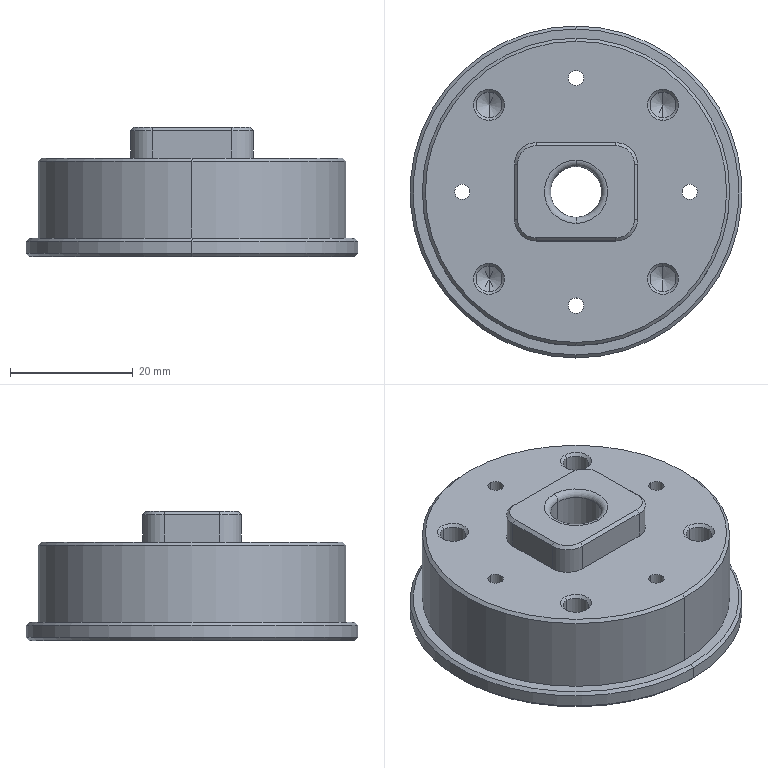Part | 1 solid | 211 faces | box 54 x 54 x 21 mm | volume 18971 mm3 | cylinder 79 | cone 77 | plane 51 | torus 4 | commonest cylinder face diameters 6 x32 28 x9 2.5 x8 4 x8 4.2 x8 7 x4